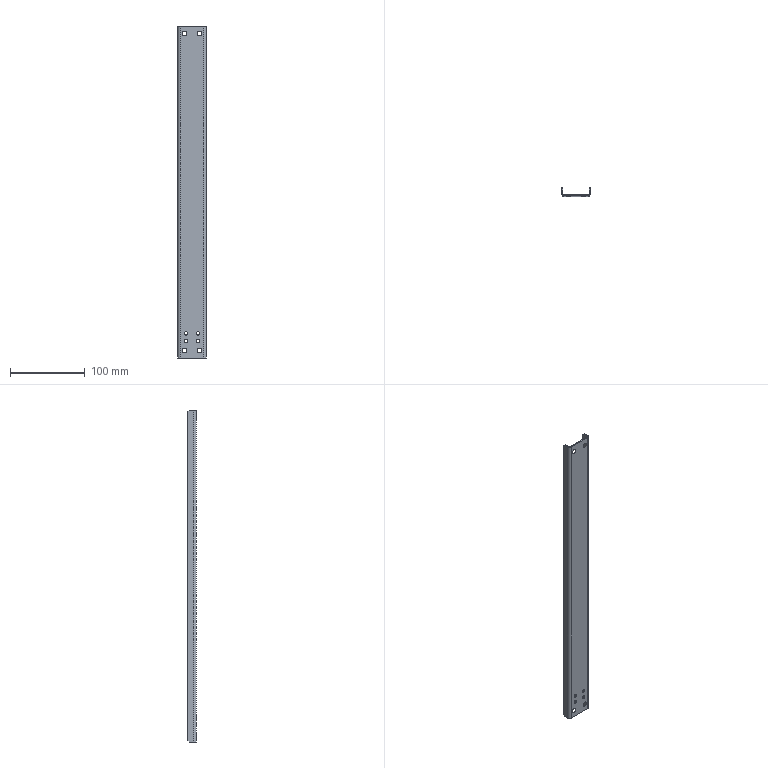Part | STEP file | 1 solid | 34 faces | box 38 x 11.5 x 445 mm | volume 36734 mm3 | plane 14 | cylinder 12 | cone 8 | commonest cylinder face diameters 4.5 x8 4 x2 7 x2